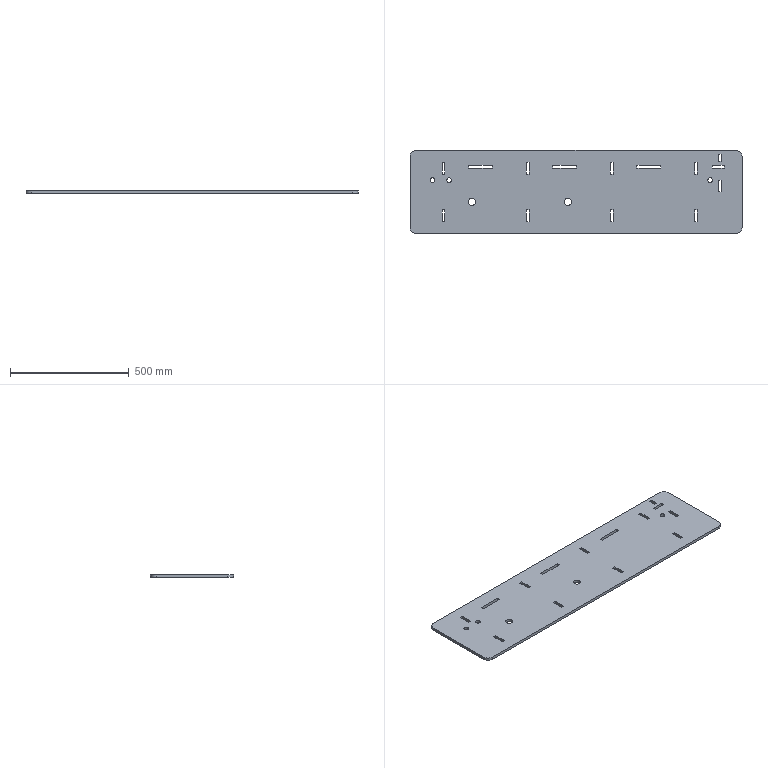Part | SolidWorks | features Fillet 1, FlatPattern 1, SMBaseFlange 1, SheetMetal 1 | 1 solid | 76 faces | box 1400 x 350 x 12 mm | volume 5725768 mm3 | plane 62 | cylinder 14 | commonest cylinder face diameters 20 x6 30 x4 50 x4